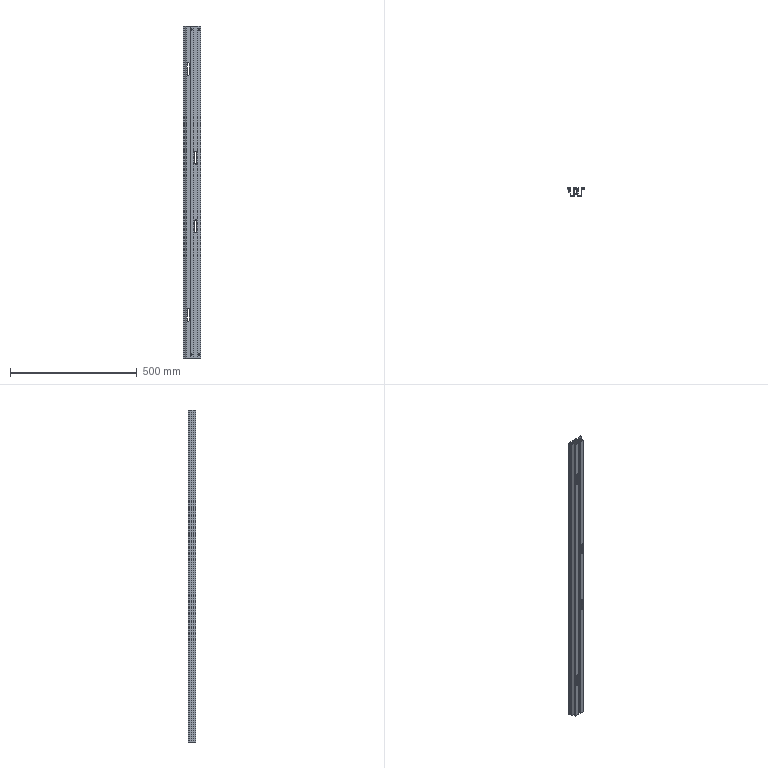Part | 1 solid | 112 faces | box 70 x 29.5 x 1310 mm | volume 471967 mm3 | plane 70 | cylinder 42 | commonest cylinder face diameters 6 x14 9 x12 2 x9 3 x7